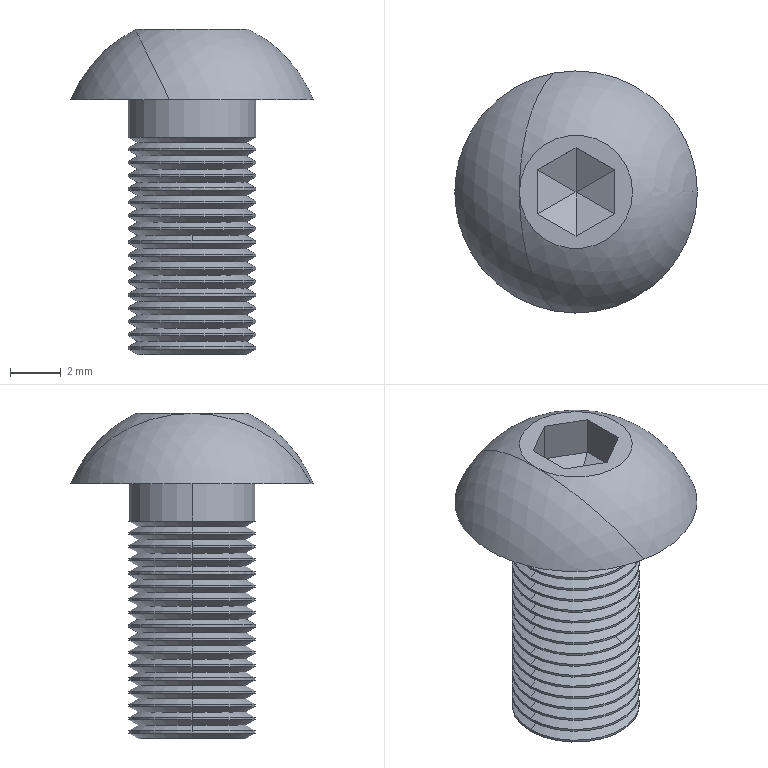Part | SolidWorks | features BaseBody 1 | 1 solid | 117 faces | box 9.5 x 9.5 x 12.75 mm | volume 291.612 mm3 | cone 66 | cylinder 34 | plane 15 | sphere 2 | commonest cylinder face diameters 5 x34